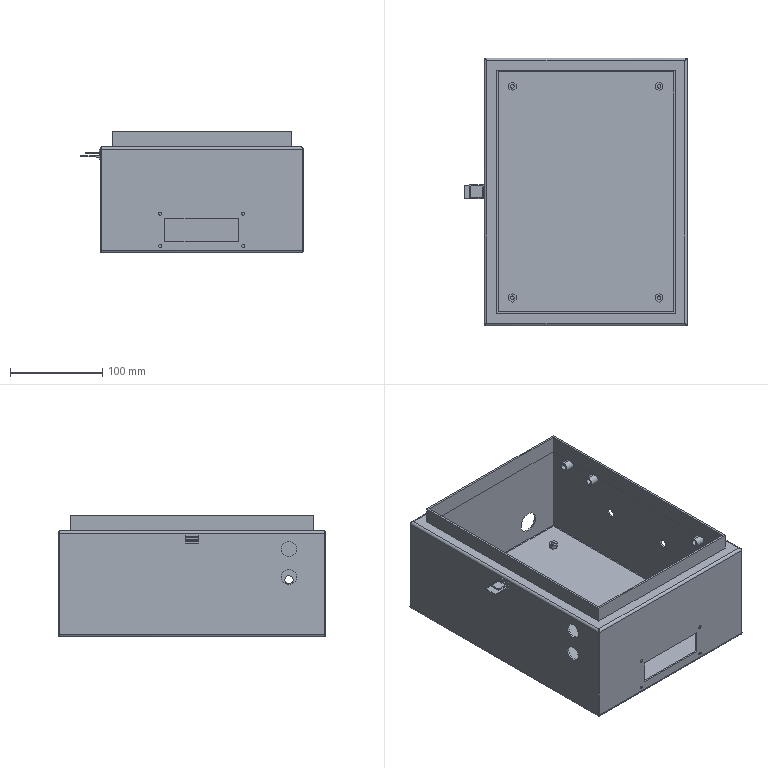Part | STEP file | Upper control box 1 | 1 solid | 188 faces | box 241 x 290 x 131.995 mm | volume 409280 mm3 | plane 92 | cylinder 88 | spline 8 | commonest cylinder face diameters 3.3 x16 6 x12 10 x12 1.473 x8 4 x8 5.473 x8